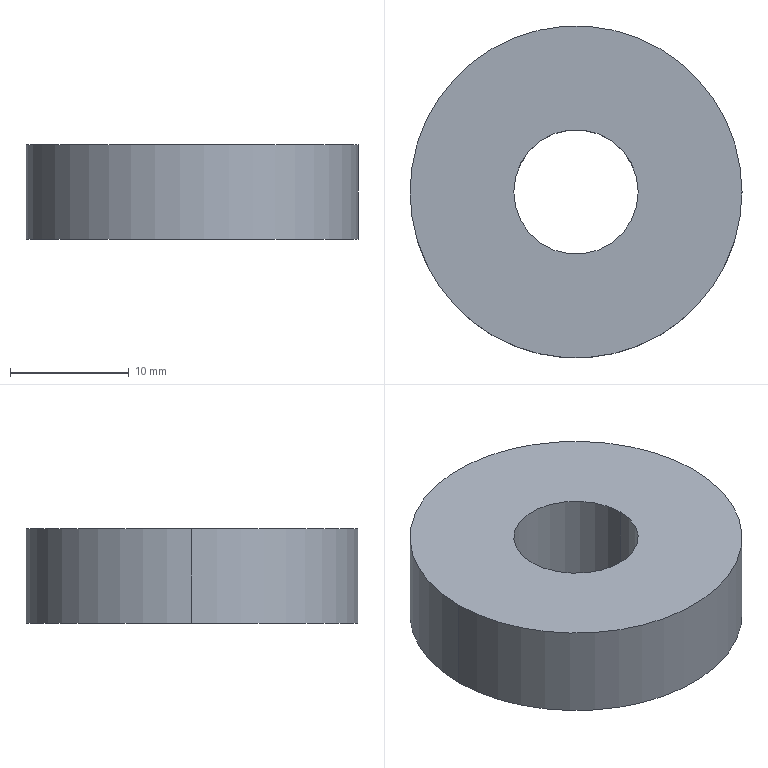Part | STEP file | bac 10.5-28 | 1 solid | 6 faces | box 28 x 28 x 8 mm | volume 4233 mm3 | cylinder 4 | plane 2 | commonest cylinder face diameters 10.5 x2 28 x2
STEP:
#1=CARTESIAN_POINT('',(0.,0.,0.));
#2=DIRECTION('',(0.,0.,1.));
#3=DIRECTION('',(1.,0.,0.));
#4=AXIS2_PLACEMENT_3D('',#1,#2,#3);
#5=CARTESIAN_POINT('',(14.,0.,0.));
#6=VERTEX_POINT('',#5);
#7=CARTESIAN_POINT('',(-14.,0.,0.));
#8=VERTEX_POINT('',#7);
#9=CARTESIAN_POINT('',(0.,0.,0.));
#10=DIRECTION('',(0.,0.,1.));
#11=DIRECTION('',(1.,0.,0.));
#12=AXIS2_PLACEMENT_3D('',#9,#10,#11);
#13=CIRCLE('',#12,14.);
#14=CARTESIAN_POINT('',(0.,0.,0.));
#15=DIRECTION('',(0.,0.,1.));
#16=DIRECTION('',(1.,0.,0.));
#17=AXIS2_PLACEMENT_3D('',#14,#15,#16);
#18=CYLINDRICAL_SURFACE('',#17,14.);
#19=CARTESIAN_POINT('',(0.,0.));
#20=DIRECTION('',(1.,0.));
#21=VECTOR('',#20,1.);
#22=LINE('',#19,#21);
#23=(GEOMETRIC_REPRESENTATION_CONTEXT(2)PARAMETRIC_REPRESENTATION_CONTEXT()REPRESENTATION_CONTEXT('',''));
#24=DEFINITIONAL_REPRESENTATION('',(#22),#23);
#25=PCURVE('',#18,#24);
#26=CARTESIAN_POINT('',(0.,0.,0.));
#27=DIRECTION('',(0.,0.,-1.));
#28=DIRECTION('',(-1.,0.,0.));
#29=AXIS2_PLACEMENT_3D('',#26,#27,#28);
#30=PLANE('',#29);
#31=CARTESIAN_POINT('',(-14.,0.));
#32=CARTESIAN_POINT('',(-14.,24.249));
#33=CARTESIAN_POINT('',(7.,12.124));
#34=CARTESIAN_POINT('',(28.,0.));
#35=CARTESIAN_POINT('',(7.,-12.124));
#36=CARTESIAN_POINT('',(-14.,-24.249));
#37=CARTESIAN_POINT('',(-14.,0.));
#38=(BOUNDED_CURVE()B_SPLINE_CURVE(2,(#31,#32,#33,#34,#35,#36,#37),.UNSPECIFIED.,.T.,.F.)B_SPLINE_CURVE_WITH_KNOTS((1,2,2,2,2,1),(-2.094,0.,2.094,4.189,6.283,8.378),.UNSPECIFIED.)CURVE()GEOMETRIC_REPRESENTATION_ITEM()RATIONAL_B_SPLINE_CURVE((1.,0.5,1.,0.5,1.,0.5,1.))REPRESENTATION_ITEM(''));
#39=(GEOMETRIC_REPRESENTATION_CONTEXT(2)PARAMETRIC_REPRESENTATION_CONTEXT()REPRESENTATION_CONTEXT('',''));
#40=DEFINITIONAL_REPRESENTATION('',(#38),#39);
#41=PCURVE('',#30,#40);
#42=SURFACE_CURVE('',#13,(#25,#41),.PCURVE_S1.);
#43=EDGE_CURVE('',#6,#8,#42,.T.);
#44=ORIENTED_EDGE('',*,*,#43,.T.);
#45=CARTESIAN_POINT('',(-14.,0.,8.));
#46=VERTEX_POINT('',#45);
#47=CARTESIAN_POINT('',(-14.,0.,0.));
#48=DIRECTION('',(0.,0.,1.));
#49=VECTOR('',#48,1.);
#50=LINE('',#47,#49);
#51=CARTESIAN_POINT('',(3.142,0.));
#52=DIRECTION('',(0.,1.));
#53=VECTOR('',#52,1.);
#54=LINE('',#51,#53);
#55=(GEOMETRIC_REPRESENTATION_CONTEXT(2)PARAMETRIC_REPRESENTATION_CONTEXT()REPRESENTATION_CONTEXT('',''));
#56=DEFINITIONAL_REPRESENTATION('',(#54),#55);
#57=PCURVE('',#18,#56);
#58=CARTESIAN_POINT('',(0.,0.,0.));
#59=DIRECTION('',(0.,0.,1.));
#60=DIRECTION('',(1.,0.,0.));
#61=AXIS2_PLACEMENT_3D('',#58,#59,#60);
#62=CYLINDRICAL_SURFACE('',#61,14.);
#63=CARTESIAN_POINT('',(3.142,0.));
#64=DIRECTION('',(0.,1.));
#65=VECTOR('',#64,1.);
#66=LINE('',#63,#65);
#67=(GEOMETRIC_REPRESENTATION_CONTEXT(2)PARAMETRIC_REPRESENTATION_CONTEXT()REPRESENTATION_CONTEXT('',''));
#68=DEFINITIONAL_REPRESENTATION('',(#66),#67);
#69=PCURVE('',#62,#68);
#70=SURFACE_CURVE('',#50,(#57,#69),.PCURVE_S1.);
#71=EDGE_CURVE('',#8,#46,#70,.T.);
#72=ORIENTED_EDGE('',*,*,#71,.T.);
#73=CARTESIAN_POINT('',(14.,0.,8.));
#74=VERTEX_POINT('',#73);
#75=CARTESIAN_POINT('',(0.,0.,8.));
#76=DIRECTION('',(0.,0.,-1.));
#77=DIRECTION('',(1.,0.,0.));
#78=AXIS2_PLACEMENT_3D('',#75,#76,#77);
#79=CIRCLE('',#78,14.);
#80=CARTESIAN_POINT('',(6.283,8.));
#81=DIRECTION('',(-1.,0.));
#82=VECTOR('',#81,1.);
#83=LINE('',#80,#82);
#84=(GEOMETRIC_REPRESENTATION_CONTEXT(2)PARAMETRIC_REPRESENTATION_CONTEXT()REPRESENTATION_CONTEXT('',''));
#85=DEFINITIONAL_REPRESENTATION('',(#83),#84);
#86=PCURVE('',#18,#85);
#87=CARTESIAN_POINT('',(0.,0.,8.));
#88=DIRECTION('',(0.,0.,-1.));
#89=DIRECTION('',(-1.,0.,0.));
#90=AXIS2_PLACEMENT_3D('',#87,#88,#89);
#91=PLANE('',#90);
#92=CARTESIAN_POINT('',(0.,0.));
#93=DIRECTION('',(-1.,0.));
#94=AXIS2_PLACEMENT_2D('',#92,#93);
#95=CIRCLE('',#94,14.);
#96=(GEOMETRIC_REPRESENTATION_CONTEXT(2)PARAMETRIC_REPRESENTATION_CONTEXT()REPRESENTATION_CONTEXT('',''));
#97=DEFINITIONAL_REPRESENTATION('',(#95),#96);
#98=PCURVE('',#91,#97);
#99=SURFACE_CURVE('',#79,(#86,#98),.PCURVE_S1.);
#100=EDGE_CURVE('',#46,#74,#99,.T.);
#101=ORIENTED_EDGE('',*,*,#100,.T.);
#102=CARTESIAN_POINT('',(14.,0.,0.));
#103=DIRECTION('',(0.,0.,1.));
#104=VECTOR('',#103,1.);
#105=LINE('',#102,#104);
#106=CARTESIAN_POINT('',(0.,0.));
#107=DIRECTION('',(0.,1.));
#108=VECTOR('',#107,1.);
#109=LINE('',#106,#108);
#110=(GEOMETRIC_REPRESENTATION_CONTEXT(2)PARAMETRIC_REPRESENTATION_CONTEXT()REPRESENTATION_CONTEXT('',''));
#111=DEFINITIONAL_REPRESENTATION('',(#109),#110);
#112=PCURVE('',#18,#111);
#113=CARTESIAN_POINT('',(6.283,0.));
#114=DIRECTION('',(0.,1.));
#115=VECTOR('',#114,1.);
#116=LINE('',#113,#115);
#117=(GEOMETRIC_REPRESENTATION_CONTEXT(2)PARAMETRIC_REPRESENTATION_CONTEXT()REPRESENTATION_CONTEXT('',''));
#118=DEFINITIONAL_REPRESENTATION('',(#116),#117);
#119=PCURVE('',#62,#118);
#120=SURFACE_CURVE('',#105,(#112,#119),.PCURVE_S1.);
#121=EDGE_CURVE('',#6,#74,#120,.T.);
#122=ORIENTED_EDGE('',*,*,#121,.F.);
#123=EDGE_LOOP('',(#44,#72,#101,#122));
#124=FACE_BOUND('',#123,.T.);
#125=ADVANCED_FACE('',(#124),#18,.T.);
#126=CARTESIAN_POINT('',(5.25,0.,0.));
#127=VERTEX_POINT('',#126);
#128=CARTESIAN_POINT('',(5.25,0.,8.));
#129=VERTEX_POINT('',#128);
#130=CARTESIAN_POINT('',(5.25,0.,0.));
#131=DIRECTION('',(0.,0.,1.));
#132=VECTOR('',#131,1.);
#133=LINE('',#130,#132);
#134=CARTESIAN_POINT('',(0.,0.,0.));
#135=DIRECTION('',(0.,0.,1.));
#136=DIRECTION('',(1.,0.,0.));
#137=AXIS2_PLACEMENT_3D('',#134,#135,#136);
#138=CYLINDRICAL_SURFACE('',#137,5.25);
#139=CARTESIAN_POINT('',(6.283,0.));
#140=DIRECTION('',(0.,1.));
#141=VECTOR('',#140,1.);
#142=LINE('',#139,#141);
#143=(GEOMETRIC_REPRESENTATION_CONTEXT(2)PARAMETRIC_REPRESENTATION_CONTEXT()REPRESENTATION_CONTEXT('',''));
#144=DEFINITIONAL_REPRESENTATION('',(#142),#143);
#145=PCURVE('',#138,#144);
#146=CARTESIAN_POINT('',(0.,0.,0.));
#147=DIRECTION('',(0.,0.,1.));
#148=DIRECTION('',(1.,0.,0.));
#149=AXIS2_PLACEMENT_3D('',#146,#147,#148);
#150=CYLINDRICAL_SURFACE('',#149,5.25);
#151=CARTESIAN_POINT('',(0.,0.));
#152=DIRECTION('',(0.,1.));
#153=VECTOR('',#152,1.);
#154=LINE('',#151,#153);
#155=(GEOMETRIC_REPRESENTATION_CONTEXT(2)PARAMETRIC_REPRESENTATION_CONTEXT()REPRESENTATION_CONTEXT('',''));
#156=DEFINITIONAL_REPRESENTATION('',(#154),#155);
#157=PCURVE('',#150,#156);
#158=SURFACE_CURVE('',#133,(#145,#157),.PCURVE_S1.);
#159=EDGE_CURVE('',#127,#129,#158,.T.);
#160=ORIENTED_EDGE('',*,*,#159,.T.);
#161=CARTESIAN_POINT('',(-5.25,0.,8.));
#162=VERTEX_POINT('',#161);
#163=CARTESIAN_POINT('',(0.,0.,8.));
#164=DIRECTION('',(0.,0.,1.));
#165=DIRECTION('',(1.,0.,0.));
#166=AXIS2_PLACEMENT_3D('',#163,#164,#165);
#167=CIRCLE('',#166,5.25);
#168=CARTESIAN_POINT('',(0.,8.));
#169=DIRECTION('',(1.,0.));
#170=VECTOR('',#169,1.);
#171=LINE('',#168,#170);
#172=(GEOMETRIC_REPRESENTATION_CONTEXT(2)PARAMETRIC_REPRESENTATION_CONTEXT()REPRESENTATION_CONTEXT('',''));
#173=DEFINITIONAL_REPRESENTATION('',(#171),#172);
#174=PCURVE('',#138,#173);
#175=CARTESIAN_POINT('',(-5.25,0.));
#176=CARTESIAN_POINT('',(-5.25,9.093));
#177=CARTESIAN_POINT('',(2.625,4.547));
#178=CARTESIAN_POINT('',(10.5,0.));
#179=CARTESIAN_POINT('',(2.625,-4.547));
#180=CARTESIAN_POINT('',(-5.25,-9.093));
#181=CARTESIAN_POINT('',(-5.25,0.));
#182=(BOUNDED_CURVE()B_SPLINE_CURVE(2,(#175,#176,#177,#178,#179,#180,#181),.UNSPECIFIED.,.T.,.F.)B_SPLINE_CURVE_WITH_KNOTS((1,2,2,2,2,1),(-2.094,0.,2.094,4.189,6.283,8.378),.UNSPECIFIED.)CURVE()GEOMETRIC_REPRESENTATION_ITEM()RATIONAL_B_SPLINE_CURVE((1.,0.5,1.,0.5,1.,0.5,1.))REPRESENTATION_ITEM(''));
#183=(GEOMETRIC_REPRESENTATION_CONTEXT(2)PARAMETRIC_REPRESENTATION_CONTEXT()REPRESENTATION_CONTEXT('',''));
#184=DEFINITIONAL_REPRESENTATION('',(#182),#183);
#185=PCURVE('',#91,#184);
#186=SURFACE_CURVE('',#167,(#174,#185),.PCURVE_S1.);
#187=EDGE_CURVE('',#162,#129,#186,.T.);
#188=ORIENTED_EDGE('',*,*,#187,.F.);
#189=CARTESIAN_POINT('',(-5.25,0.,0.));
#190=VERTEX_POINT('',#189);
#191=CARTESIAN_POINT('',(-5.25,0.,0.));
#192=DIRECTION('',(0.,0.,1.));
#193=VECTOR('',#192,1.);
#194=LINE('',#191,#193);
#195=CARTESIAN_POINT('',(3.142,0.));
#196=DIRECTION('',(0.,1.));
#197=VECTOR('',#196,1.);
#198=LINE('',#195,#197);
#199=(GEOMETRIC_REPRESENTATION_CONTEXT(2)PARAMETRIC_REPRESENTATION_CONTEXT()REPRESENTATION_CONTEXT('',''));
#200=DEFINITIONAL_REPRESENTATION('',(#198),#199);
#201=PCURVE('',#138,#200);
#202=CARTESIAN_POINT('',(3.142,0.));
#203=DIRECTION('',(0.,1.));
#204=VECTOR('',#203,1.);
#205=LINE('',#202,#204);
#206=(GEOMETRIC_REPRESENTATION_CONTEXT(2)PARAMETRIC_REPRESENTATION_CONTEXT()REPRESENTATION_CONTEXT('',''));
#207=DEFINITIONAL_REPRESENTATION('',(#205),#206);
#208=PCURVE('',#150,#207);
#209=SURFACE_CURVE('',#194,(#201,#208),.PCURVE_S1.);
#210=EDGE_CURVE('',#190,#162,#209,.T.);
#211=ORIENTED_EDGE('',*,*,#210,.F.);
#212=CARTESIAN_POINT('',(0.,0.,0.));
#213=DIRECTION('',(0.,0.,1.));
#214=DIRECTION('',(1.,0.,0.));
#215=AXIS2_PLACEMENT_3D('',#212,#213,#214);
#216=CIRCLE('',#215,5.25);
#217=CARTESIAN_POINT('',(0.,0.));
#218=DIRECTION('',(1.,0.));
#219=VECTOR('',#218,1.);
#220=LINE('',#217,#219);
#221=(GEOMETRIC_REPRESENTATION_CONTEXT(2)PARAMETRIC_REPRESENTATION_CONTEXT()REPRESENTATION_CONTEXT('',''));
#222=DEFINITIONAL_REPRESENTATION('',(#220),#221);
#223=PCURVE('',#138,#222);
#224=CARTESIAN_POINT('',(-5.25,0.));
#225=CARTESIAN_POINT('',(-5.25,9.093));
#226=CARTESIAN_POINT('',(2.625,4.547));
#227=CARTESIAN_POINT('',(10.5,0.));
#228=CARTESIAN_POINT('',(2.625,-4.547));
#229=CARTESIAN_POINT('',(-5.25,-9.093));
#230=CARTESIAN_POINT('',(-5.25,0.));
#231=(BOUNDED_CURVE()B_SPLINE_CURVE(2,(#224,#225,#226,#227,#228,#229,#230),.UNSPECIFIED.,.T.,.F.)B_SPLINE_CURVE_WITH_KNOTS((1,2,2,2,2,1),(-2.094,0.,2.094,4.189,6.283,8.378),.UNSPECIFIED.)CURVE()GEOMETRIC_REPRESENTATION_ITEM()RATIONAL_B_SPLINE_CURVE((1.,0.5,1.,0.5,1.,0.5,1.))REPRESENTATION_ITEM(''));
#232=(GEOMETRIC_REPRESENTATION_CONTEXT(2)PARAMETRIC_REPRESENTATION_CONTEXT()REPRESENTATION_CONTEXT('',''));
#233=DEFINITIONAL_REPRESENTATION('',(#231),#232);
#234=PCURVE('',#30,#233);
#235=SURFACE_CURVE('',#216,(#223,#234),.PCURVE_S1.);
#236=EDGE_CURVE('',#190,#127,#235,.T.);
#237=ORIENTED_EDGE('',*,*,#236,.T.);
#238=EDGE_LOOP('',(#160,#188,#211,#237));
#239=FACE_BOUND('',#238,.F.);
#240=ADVANCED_FACE('',(#239),#138,.F.);
#241=ORIENTED_EDGE('',*,*,#71,.F.);
#242=CARTESIAN_POINT('',(0.,0.,0.));
#243=DIRECTION('',(0.,0.,1.));
#244=DIRECTION('',(1.,0.,0.));
#245=AXIS2_PLACEMENT_3D('',#242,#243,#244);
#246=CIRCLE('',#245,14.);
#247=CARTESIAN_POINT('',(0.,0.));
#248=DIRECTION('',(1.,0.));
#249=VECTOR('',#248,1.);
#250=LINE('',#247,#249);
#251=(GEOMETRIC_REPRESENTATION_CONTEXT(2)PARAMETRIC_REPRESENTATION_CONTEXT()REPRESENTATION_CONTEXT('',''));
#252=DEFINITIONAL_REPRESENTATION('',(#250),#251);
#253=PCURVE('',#62,#252);
#254=CARTESIAN_POINT('',(-14.,0.));
#255=CARTESIAN_POINT('',(-14.,24.249));
#256=CARTESIAN_POINT('',(7.,12.124));
#257=CARTESIAN_POINT('',(28.,0.));
#258=CARTESIAN_POINT('',(7.,-12.124));
#259=CARTESIAN_POINT('',(-14.,-24.249));
#260=CARTESIAN_POINT('',(-14.,0.));
#261=(BOUNDED_CURVE()B_SPLINE_CURVE(2,(#254,#255,#256,#257,#258,#259,#260),.UNSPECIFIED.,.T.,.F.)B_SPLINE_CURVE_WITH_KNOTS((1,2,2,2,2,1),(-2.094,0.,2.094,4.189,6.283,8.378),.UNSPECIFIED.)CURVE()GEOMETRIC_REPRESENTATION_ITEM()RATIONAL_B_SPLINE_CURVE((1.,0.5,1.,0.5,1.,0.5,1.))REPRESENTATION_ITEM(''));
#262=(GEOMETRIC_REPRESENTATION_CONTEXT(2)PARAMETRIC_REPRESENTATION_CONTEXT()REPRESENTATION_CONTEXT('',''));
#263=DEFINITIONAL_REPRESENTATION('',(#261),#262);
#264=PCURVE('',#30,#263);
#265=SURFACE_CURVE('',#246,(#253,#264),.PCURVE_S1.);
#266=EDGE_CURVE('',#8,#6,#265,.T.);
#267=ORIENTED_EDGE('',*,*,#266,.T.);
#268=ORIENTED_EDGE('',*,*,#121,.T.);
#269=CARTESIAN_POINT('',(0.,0.,8.));
#270=DIRECTION('',(0.,0.,-1.));
#271=DIRECTION('',(1.,0.,0.));
#272=AXIS2_PLACEMENT_3D('',#269,#270,#271);
#273=CIRCLE('',#272,14.);
#274=CARTESIAN_POINT('',(6.283,8.));
#275=DIRECTION('',(-1.,0.));
#276=VECTOR('',#275,1.);
#277=LINE('',#274,#276);
#278=(GEOMETRIC_REPRESENTATION_CONTEXT(2)PARAMETRIC_REPRESENTATION_CONTEXT()REPRESENTATION_CONTEXT('',''));
#279=DEFINITIONAL_REPRESENTATION('',(#277),#278);
#280=PCURVE('',#62,#279);
#281=CARTESIAN_POINT('',(0.,0.));
#282=DIRECTION('',(-1.,0.));
#283=AXIS2_PLACEMENT_2D('',#281,#282);
#284=CIRCLE('',#283,14.);
#285=(GEOMETRIC_REPRESENTATION_CONTEXT(2)PARAMETRIC_REPRESENTATION_CONTEXT()REPRESENTATION_CONTEXT('',''));
#286=DEFINITIONAL_REPRESENTATION('',(#284),#285);
#287=PCURVE('',#91,#286);
#288=SURFACE_CURVE('',#273,(#280,#287),.PCURVE_S1.);
#289=EDGE_CURVE('',#74,#46,#288,.T.);
#290=ORIENTED_EDGE('',*,*,#289,.T.);
#291=EDGE_LOOP('',(#241,#267,#268,#290));
#292=FACE_BOUND('',#291,.T.);
#293=ADVANCED_FACE('',(#292),#62,.T.);
#294=CARTESIAN_POINT('',(0.,0.,0.));
#295=DIRECTION('',(0.,0.,1.));
#296=DIRECTION('',(1.,0.,0.));
#297=AXIS2_PLACEMENT_3D('',#294,#295,#296);
#298=CIRCLE('',#297,5.25);
#299=CARTESIAN_POINT('',(-5.25,0.));
#300=CARTESIAN_POINT('',(-5.25,9.093));
#301=CARTESIAN_POINT('',(2.625,4.547));
#302=CARTESIAN_POINT('',(10.5,0.));
#303=CARTESIAN_POINT('',(2.625,-4.547));
#304=CARTESIAN_POINT('',(-5.25,-9.093));
#305=CARTESIAN_POINT('',(-5.25,0.));
#306=(BOUNDED_CURVE()B_SPLINE_CURVE(2,(#299,#300,#301,#302,#303,#304,#305),.UNSPECIFIED.,.T.,.F.)B_SPLINE_CURVE_WITH_KNOTS((1,2,2,2,2,1),(-2.094,0.,2.094,4.189,6.283,8.378),.UNSPECIFIED.)CURVE()GEOMETRIC_REPRESENTATION_ITEM()RATIONAL_B_SPLINE_CURVE((1.,0.5,1.,0.5,1.,0.5,1.))REPRESENTATION_ITEM(''));
#307=(GEOMETRIC_REPRESENTATION_CONTEXT(2)PARAMETRIC_REPRESENTATION_CONTEXT()REPRESENTATION_CONTEXT('',''));
#308=DEFINITIONAL_REPRESENTATION('',(#306),#307);
#309=PCURVE('',#30,#308);
#310=CARTESIAN_POINT('',(0.,0.));
#311=DIRECTION('',(1.,0.));
#312=VECTOR('',#311,1.);
#313=LINE('',#310,#312);
#314=(GEOMETRIC_REPRESENTATION_CONTEXT(2)PARAMETRIC_REPRESENTATION_CONTEXT()REPRESENTATION_CONTEXT('',''));
#315=DEFINITIONAL_REPRESENTATION('',(#313),#314);
#316=PCURVE('',#150,#315);
#317=SURFACE_CURVE('',#298,(#309,#316),.PCURVE_S1.);
#318=EDGE_CURVE('',#127,#190,#317,.T.);
#319=ORIENTED_EDGE('',*,*,#318,.T.);
#320=ORIENTED_EDGE('',*,*,#236,.T.);
#321=EDGE_LOOP('',(#319,#320));
#322=FACE_BOUND('',#321,.T.);
#323=ORIENTED_EDGE('',*,*,#43,.F.);
#324=ORIENTED_EDGE('',*,*,#266,.F.);
#325=EDGE_LOOP('',(#323,#324));
#326=FACE_BOUND('',#325,.T.);
#327=ADVANCED_FACE('',(#322,#326),#30,.T.);
#328=CARTESIAN_POINT('',(0.,0.,8.));
#329=DIRECTION('',(0.,0.,1.));
#330=DIRECTION('',(1.,0.,0.));
#331=AXIS2_PLACEMENT_3D('',#328,#329,#330);
#332=CIRCLE('',#331,5.25);
#333=CARTESIAN_POINT('',(-5.25,0.));
#334=CARTESIAN_POINT('',(-5.25,9.093));
#335=CARTESIAN_POINT('',(2.625,4.547));
#336=CARTESIAN_POINT('',(10.5,0.));
#337=CARTESIAN_POINT('',(2.625,-4.547));
#338=CARTESIAN_POINT('',(-5.25,-9.093));
#339=CARTESIAN_POINT('',(-5.25,0.));
#340=(BOUNDED_CURVE()B_SPLINE_CURVE(2,(#333,#334,#335,#336,#337,#338,#339),.UNSPECIFIED.,.T.,.F.)B_SPLINE_CURVE_WITH_KNOTS((1,2,2,2,2,1),(-2.094,0.,2.094,4.189,6.283,8.378),.UNSPECIFIED.)CURVE()GEOMETRIC_REPRESENTATION_ITEM()RATIONAL_B_SPLINE_CURVE((1.,0.5,1.,0.5,1.,0.5,1.))REPRESENTATION_ITEM(''));
#341=(GEOMETRIC_REPRESENTATION_CONTEXT(2)PARAMETRIC_REPRESENTATION_CONTEXT()REPRESENTATION_CONTEXT('',''));
#342=DEFINITIONAL_REPRESENTATION('',(#340),#341);
#343=PCURVE('',#91,#342);
#344=CARTESIAN_POINT('',(0.,8.));
#345=DIRECTION('',(1.,0.));
#346=VECTOR('',#345,1.);
#347=LINE('',#344,#346);
#348=(GEOMETRIC_REPRESENTATION_CONTEXT(2)PARAMETRIC_REPRESENTATION_CONTEXT()REPRESENTATION_CONTEXT('',''));
#349=DEFINITIONAL_REPRESENTATION('',(#347),#348);
#350=PCURVE('',#150,#349);
#351=SURFACE_CURVE('',#332,(#343,#350),.PCURVE_S1.);
#352=EDGE_CURVE('',#129,#162,#351,.T.);
#353=ORIENTED_EDGE('',*,*,#352,.F.);
#354=ORIENTED_EDGE('',*,*,#187,.F.);
#355=EDGE_LOOP('',(#353,#354));
#356=FACE_BOUND('',#355,.T.);
#357=ORIENTED_EDGE('',*,*,#289,.F.);
#358=ORIENTED_EDGE('',*,*,#100,.F.);
#359=EDGE_LOOP('',(#357,#358));
#360=FACE_BOUND('',#359,.T.);
#361=ADVANCED_FACE('',(#356,#360),#91,.F.);
#362=ORIENTED_EDGE('',*,*,#352,.F.);
#363=ORIENTED_EDGE('',*,*,#159,.F.);
#364=ORIENTED_EDGE('',*,*,#318,.T.);
#365=ORIENTED_EDGE('',*,*,#210,.T.);
#366=EDGE_LOOP('',(#362,#363,#364,#365));
#367=FACE_BOUND('',#366,.F.);
#368=ADVANCED_FACE('',(#367),#150,.F.);
#369=CLOSED_SHELL('',(#125,#240,#293,#327,#361,#368));
#370=MANIFOLD_SOLID_BREP('',#369);
#371=(LENGTH_UNIT()NAMED_UNIT(*)SI_UNIT(.MILLI.,.METRE.));
#372=UNCERTAINTY_MEASURE_WITH_UNIT(LENGTH_MEASURE(0.0000001),#371,'','');
#373=(NAMED_UNIT(*)PLANE_ANGLE_UNIT()SI_UNIT($,.RADIAN.));
#374=(NAMED_UNIT(*)SI_UNIT($,.STERADIAN.)SOLID_ANGLE_UNIT());
#375=(GEOMETRIC_REPRESENTATION_CONTEXT(3)GLOBAL_UNCERTAINTY_ASSIGNED_CONTEXT((#372))GLOBAL_UNIT_ASSIGNED_CONTEXT((#371,#373,#374))REPRESENTATION_CONTEXT('',''));
#376=ADVANCED_BREP_SHAPE_REPRESENTATION('',(#4,#370),#375);